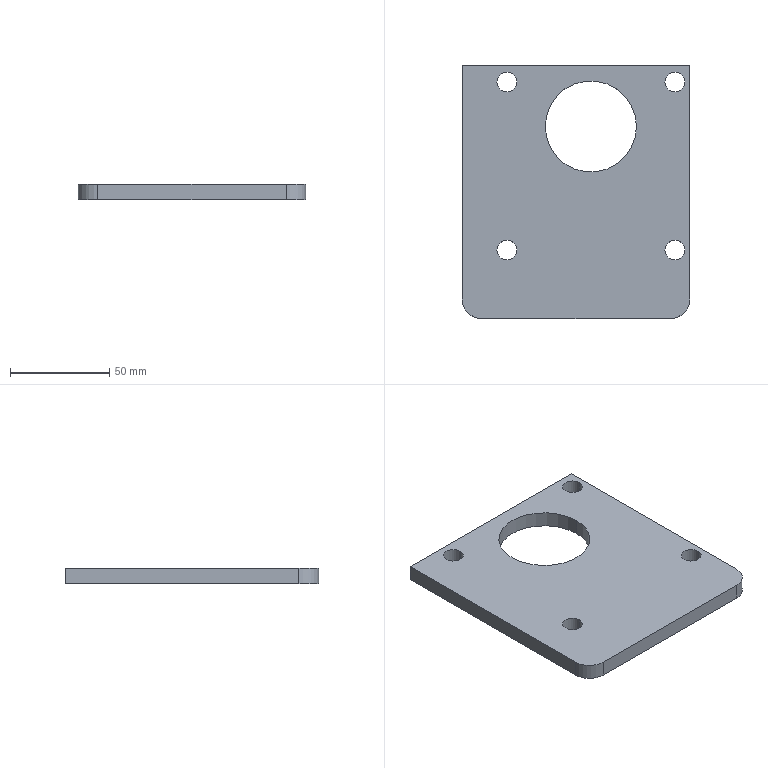Part | SolidWorks | features Chamfer 1, Extrusion 1, Fillet 1, HoleWzd 1, ICE 1 | 1 solid | 18 faces | box 115 x 128 x 8 mm | volume 101608 mm3 | cylinder 12 | plane 6 | commonest cylinder face diameters 10 x8 20 x2 46 x2
STEP:
#1=CARTESIAN_POINT('',(30.5,33.074,-4.));
#2=VERTEX_POINT('',#1);
#3=CARTESIAN_POINT('',(-15.5,33.074,-4.));
#4=VERTEX_POINT('',#3);
#5=CARTESIAN_POINT('',(7.5,33.074,-4.));
#6=DIRECTION('',(0.,0.,-1.));
#7=DIRECTION('',(1.,0.,0.));
#8=AXIS2_PLACEMENT_3D('',#5,#6,#7);
#9=CIRCLE('',#8,23.);
#10=EDGE_CURVE('',#2,#4,#9,.T.);
#11=ORIENTED_EDGE('',*,*,#10,.T.);
#12=CARTESIAN_POINT('',(-15.5,33.074,4.));
#13=VERTEX_POINT('',#12);
#14=CARTESIAN_POINT('',(-15.5,33.074,-4.001));
#15=DIRECTION('',(0.,0.,1.));
#16=VECTOR('',#15,1000.);
#17=LINE('',#14,#16);
#18=EDGE_CURVE('',#4,#13,#17,.T.);
#19=ORIENTED_EDGE('',*,*,#18,.T.);
#20=CARTESIAN_POINT('',(30.5,33.074,4.));
#21=VERTEX_POINT('',#20);
#22=CARTESIAN_POINT('',(7.5,33.074,4.));
#23=DIRECTION('',(0.,0.,1.));
#24=DIRECTION('',(1.,0.,0.));
#25=AXIS2_PLACEMENT_3D('',#22,#23,#24);
#26=CIRCLE('',#25,23.);
#27=EDGE_CURVE('',#13,#21,#26,.T.);
#28=ORIENTED_EDGE('',*,*,#27,.T.);
#29=CARTESIAN_POINT('',(30.5,33.074,-4.001));
#30=DIRECTION('',(0.,0.,1.));
#31=VECTOR('',#30,1000.);
#32=LINE('',#29,#31);
#33=EDGE_CURVE('',#2,#21,#32,.T.);
#34=ORIENTED_EDGE('',*,*,#33,.F.);
#35=EDGE_LOOP('',(#11,#19,#28,#34));
#36=FACE_OUTER_BOUND('',#35,.T.);
#37=CARTESIAN_POINT('',(7.5,33.074,-4.001));
#38=DIRECTION('',(0.,0.,1.));
#39=DIRECTION('',(1.,0.,0.));
#40=AXIS2_PLACEMENT_3D('',#37,#38,#39);
#41=CYLINDRICAL_SURFACE('',#40,23.);
#42=ADVANCED_FACE('',(#36),#41,.F.);
#43=CARTESIAN_POINT('',(-39.926,55.5,-4.));
#44=VERTEX_POINT('',#43);
#45=CARTESIAN_POINT('',(-29.926,55.5,-4.));
#46=VERTEX_POINT('',#45);
#47=CARTESIAN_POINT('',(-34.926,55.5,-4.));
#48=DIRECTION('',(0.,0.,1.));
#49=DIRECTION('',(1.,0.,0.));
#50=AXIS2_PLACEMENT_3D('',#47,#48,#49);
#51=CIRCLE('',#50,5.);
#52=EDGE_CURVE('',#44,#46,#51,.T.);
#53=ORIENTED_EDGE('',*,*,#52,.F.);
#54=CARTESIAN_POINT('',(-39.926,55.5,4.));
#55=VERTEX_POINT('',#54);
#56=CARTESIAN_POINT('',(-39.926,55.5,4.));
#57=DIRECTION('',(0.,0.,1.));
#58=VECTOR('',#57,1000.);
#59=LINE('',#56,#58);
#60=EDGE_CURVE('',#44,#55,#59,.T.);
#61=ORIENTED_EDGE('',*,*,#60,.T.);
#62=CARTESIAN_POINT('',(-29.926,55.5,4.));
#63=VERTEX_POINT('',#62);
#64=CARTESIAN_POINT('',(-34.926,55.5,4.));
#65=DIRECTION('',(0.,0.,1.));
#66=DIRECTION('',(1.,0.,0.));
#67=AXIS2_PLACEMENT_3D('',#64,#65,#66);
#68=CIRCLE('',#67,5.);
#69=EDGE_CURVE('',#55,#63,#68,.T.);
#70=ORIENTED_EDGE('',*,*,#69,.T.);
#71=CARTESIAN_POINT('',(-29.926,55.5,4.));
#72=DIRECTION('',(0.,0.,1.));
#73=VECTOR('',#72,1000.);
#74=LINE('',#71,#73);
#75=EDGE_CURVE('',#46,#63,#74,.T.);
#76=ORIENTED_EDGE('',*,*,#75,.F.);
#77=EDGE_LOOP('',(#53,#61,#70,#76));
#78=FACE_OUTER_BOUND('',#77,.T.);
#79=CARTESIAN_POINT('',(-34.926,55.5,4.));
#80=DIRECTION('',(0.,0.,1.));
#81=DIRECTION('',(1.,0.,0.));
#82=AXIS2_PLACEMENT_3D('',#79,#80,#81);
#83=CYLINDRICAL_SURFACE('',#82,5.);
#84=ADVANCED_FACE('',(#78),#83,.F.);
#85=CARTESIAN_POINT('',(44.926,55.5,-4.));
#86=VERTEX_POINT('',#85);
#87=CARTESIAN_POINT('',(54.926,55.5,-4.));
#88=VERTEX_POINT('',#87);
#89=CARTESIAN_POINT('',(49.926,55.5,-4.));
#90=DIRECTION('',(0.,0.,1.));
#91=DIRECTION('',(1.,0.,0.));
#92=AXIS2_PLACEMENT_3D('',#89,#90,#91);
#93=CIRCLE('',#92,5.);
#94=EDGE_CURVE('',#86,#88,#93,.T.);
#95=ORIENTED_EDGE('',*,*,#94,.F.);
#96=CARTESIAN_POINT('',(44.926,55.5,4.));
#97=VERTEX_POINT('',#96);
#98=CARTESIAN_POINT('',(44.926,55.5,4.));
#99=DIRECTION('',(0.,0.,1.));
#100=VECTOR('',#99,1000.);
#101=LINE('',#98,#100);
#102=EDGE_CURVE('',#86,#97,#101,.T.);
#103=ORIENTED_EDGE('',*,*,#102,.T.);
#104=CARTESIAN_POINT('',(54.926,55.5,4.));
#105=VERTEX_POINT('',#104);
#106=CARTESIAN_POINT('',(49.926,55.5,4.));
#107=DIRECTION('',(0.,0.,1.));
#108=DIRECTION('',(1.,0.,0.));
#109=AXIS2_PLACEMENT_3D('',#106,#107,#108);
#110=CIRCLE('',#109,5.);
#111=EDGE_CURVE('',#97,#105,#110,.T.);
#112=ORIENTED_EDGE('',*,*,#111,.T.);
#113=CARTESIAN_POINT('',(54.926,55.5,4.));
#114=DIRECTION('',(0.,0.,1.));
#115=VECTOR('',#114,1000.);
#116=LINE('',#113,#115);
#117=EDGE_CURVE('',#88,#105,#116,.T.);
#118=ORIENTED_EDGE('',*,*,#117,.F.);
#119=EDGE_LOOP('',(#95,#103,#112,#118));
#120=FACE_OUTER_BOUND('',#119,.T.);
#121=CARTESIAN_POINT('',(49.926,55.5,4.));
#122=DIRECTION('',(0.,0.,1.));
#123=DIRECTION('',(1.,0.,0.));
#124=AXIS2_PLACEMENT_3D('',#121,#122,#123);
#125=CYLINDRICAL_SURFACE('',#124,5.);
#126=ADVANCED_FACE('',(#120),#125,.F.);
#127=CARTESIAN_POINT('',(44.926,-29.353,-4.));
#128=VERTEX_POINT('',#127);
#129=CARTESIAN_POINT('',(54.926,-29.353,-4.));
#130=VERTEX_POINT('',#129);
#131=CARTESIAN_POINT('',(49.926,-29.353,-4.));
#132=DIRECTION('',(0.,0.,1.));
#133=DIRECTION('',(1.,0.,0.));
#134=AXIS2_PLACEMENT_3D('',#131,#132,#133);
#135=CIRCLE('',#134,5.);
#136=EDGE_CURVE('',#128,#130,#135,.T.);
#137=ORIENTED_EDGE('',*,*,#136,.F.);
#138=CARTESIAN_POINT('',(44.926,-29.353,4.));
#139=VERTEX_POINT('',#138);
#140=CARTESIAN_POINT('',(44.926,-29.353,4.));
#141=DIRECTION('',(0.,0.,1.));
#142=VECTOR('',#141,1000.);
#143=LINE('',#140,#142);
#144=EDGE_CURVE('',#128,#139,#143,.T.);
#145=ORIENTED_EDGE('',*,*,#144,.T.);
#146=CARTESIAN_POINT('',(54.926,-29.353,4.));
#147=VERTEX_POINT('',#146);
#148=CARTESIAN_POINT('',(49.926,-29.353,4.));
#149=DIRECTION('',(0.,0.,1.));
#150=DIRECTION('',(1.,0.,0.));
#151=AXIS2_PLACEMENT_3D('',#148,#149,#150);
#152=CIRCLE('',#151,5.);
#153=EDGE_CURVE('',#139,#147,#152,.T.);
#154=ORIENTED_EDGE('',*,*,#153,.T.);
#155=CARTESIAN_POINT('',(54.926,-29.353,4.));
#156=DIRECTION('',(0.,0.,1.));
#157=VECTOR('',#156,1000.);
#158=LINE('',#155,#157);
#159=EDGE_CURVE('',#130,#147,#158,.T.);
#160=ORIENTED_EDGE('',*,*,#159,.F.);
#161=EDGE_LOOP('',(#137,#145,#154,#160));
#162=FACE_OUTER_BOUND('',#161,.T.);
#163=CARTESIAN_POINT('',(49.926,-29.353,4.));
#164=DIRECTION('',(0.,0.,1.));
#165=DIRECTION('',(1.,0.,0.));
#166=AXIS2_PLACEMENT_3D('',#163,#164,#165);
#167=CYLINDRICAL_SURFACE('',#166,5.);
#168=ADVANCED_FACE('',(#162),#167,.F.);
#169=CARTESIAN_POINT('',(-39.926,-29.353,-4.));
#170=VERTEX_POINT('',#169);
#171=CARTESIAN_POINT('',(-29.926,-29.353,-4.));
#172=VERTEX_POINT('',#171);
#173=CARTESIAN_POINT('',(-34.926,-29.353,-4.));
#174=DIRECTION('',(0.,0.,1.));
#175=DIRECTION('',(1.,0.,0.));
#176=AXIS2_PLACEMENT_3D('',#173,#174,#175);
#177=CIRCLE('',#176,5.);
#178=EDGE_CURVE('',#170,#172,#177,.T.);
#179=ORIENTED_EDGE('',*,*,#178,.F.);
#180=CARTESIAN_POINT('',(-39.926,-29.353,4.));
#181=VERTEX_POINT('',#180);
#182=CARTESIAN_POINT('',(-39.926,-29.353,4.));
#183=DIRECTION('',(0.,0.,1.));
#184=VECTOR('',#183,1000.);
#185=LINE('',#182,#184);
#186=EDGE_CURVE('',#170,#181,#185,.T.);
#187=ORIENTED_EDGE('',*,*,#186,.T.);
#188=CARTESIAN_POINT('',(-29.926,-29.353,4.));
#189=VERTEX_POINT('',#188);
#190=CARTESIAN_POINT('',(-34.926,-29.353,4.));
#191=DIRECTION('',(0.,0.,1.));
#192=DIRECTION('',(1.,0.,0.));
#193=AXIS2_PLACEMENT_3D('',#190,#191,#192);
#194=CIRCLE('',#193,5.);
#195=EDGE_CURVE('',#181,#189,#194,.T.);
#196=ORIENTED_EDGE('',*,*,#195,.T.);
#197=CARTESIAN_POINT('',(-29.926,-29.353,4.));
#198=DIRECTION('',(0.,0.,1.));
#199=VECTOR('',#198,1000.);
#200=LINE('',#197,#199);
#201=EDGE_CURVE('',#172,#189,#200,.T.);
#202=ORIENTED_EDGE('',*,*,#201,.F.);
#203=EDGE_LOOP('',(#179,#187,#196,#202));
#204=FACE_OUTER_BOUND('',#203,.T.);
#205=CARTESIAN_POINT('',(-34.926,-29.353,4.));
#206=DIRECTION('',(0.,0.,1.));
#207=DIRECTION('',(1.,0.,0.));
#208=AXIS2_PLACEMENT_3D('',#205,#206,#207);
#209=CYLINDRICAL_SURFACE('',#208,5.);
#210=ADVANCED_FACE('',(#204),#209,.F.);
#211=CARTESIAN_POINT('',(-57.5,64.,-4.));
#212=VERTEX_POINT('',#211);
#213=CARTESIAN_POINT('',(-57.5,-54.,-4.));
#214=VERTEX_POINT('',#213);
#215=CARTESIAN_POINT('',(-57.5,-64.,-4.));
#216=DIRECTION('',(0.,-1.,0.));
#217=VECTOR('',#216,1000.);
#218=LINE('',#215,#217);
#219=EDGE_CURVE('',#212,#214,#218,.T.);
#220=ORIENTED_EDGE('',*,*,#219,.T.);
#221=CARTESIAN_POINT('',(-57.5,-54.,4.));
#222=VERTEX_POINT('',#221);
#223=CARTESIAN_POINT('',(-57.5,-54.,4.));
#224=DIRECTION('',(0.,0.,1.));
#225=VECTOR('',#224,1000.);
#226=LINE('',#223,#225);
#227=EDGE_CURVE('',#214,#222,#226,.T.);
#228=ORIENTED_EDGE('',*,*,#227,.T.);
#229=CARTESIAN_POINT('',(-57.5,64.,4.));
#230=VERTEX_POINT('',#229);
#231=CARTESIAN_POINT('',(-57.5,-64.,4.));
#232=DIRECTION('',(0.,-1.,0.));
#233=VECTOR('',#232,1000.);
#234=LINE('',#231,#233);
#235=EDGE_CURVE('',#230,#222,#234,.T.);
#236=ORIENTED_EDGE('',*,*,#235,.F.);
#237=CARTESIAN_POINT('',(-57.5,64.,4.));
#238=DIRECTION('',(0.,0.,-1.));
#239=VECTOR('',#238,1000.);
#240=LINE('',#237,#239);
#241=EDGE_CURVE('',#230,#212,#240,.T.);
#242=ORIENTED_EDGE('',*,*,#241,.T.);
#243=EDGE_LOOP('',(#220,#228,#236,#242));
#244=FACE_OUTER_BOUND('',#243,.T.);
#245=CARTESIAN_POINT('',(-57.5,-64.,4.));
#246=DIRECTION('',(1.,0.,0.));
#247=DIRECTION('',(0.,0.,-1.));
#248=AXIS2_PLACEMENT_3D('',#245,#246,#247);
#249=PLANE('',#248);
#250=ADVANCED_FACE('',(#244),#249,.F.);
#251=CARTESIAN_POINT('',(-47.5,-64.,-4.));
#252=VERTEX_POINT('',#251);
#253=CARTESIAN_POINT('',(47.5,-64.,-4.));
#254=VERTEX_POINT('',#253);
#255=CARTESIAN_POINT('',(57.5,-64.,-4.));
#256=DIRECTION('',(1.,0.,0.));
#257=VECTOR('',#256,1000.);
#258=LINE('',#255,#257);
#259=EDGE_CURVE('',#252,#254,#258,.T.);
#260=ORIENTED_EDGE('',*,*,#259,.T.);
#261=CARTESIAN_POINT('',(47.5,-64.,4.));
#262=VERTEX_POINT('',#261);
#263=CARTESIAN_POINT('',(47.5,-64.,4.));
#264=DIRECTION('',(0.,0.,1.));
#265=VECTOR('',#264,1000.);
#266=LINE('',#263,#265);
#267=EDGE_CURVE('',#254,#262,#266,.T.);
#268=ORIENTED_EDGE('',*,*,#267,.T.);
#269=CARTESIAN_POINT('',(-47.5,-64.,4.));
#270=VERTEX_POINT('',#269);
#271=CARTESIAN_POINT('',(57.5,-64.,4.));
#272=DIRECTION('',(1.,0.,0.));
#273=VECTOR('',#272,1000.);
#274=LINE('',#271,#273);
#275=EDGE_CURVE('',#270,#262,#274,.T.);
#276=ORIENTED_EDGE('',*,*,#275,.F.);
#277=CARTESIAN_POINT('',(-47.5,-64.,4.));
#278=DIRECTION('',(0.,0.,-1.));
#279=VECTOR('',#278,1000.);
#280=LINE('',#277,#279);
#281=EDGE_CURVE('',#270,#252,#280,.T.);
#282=ORIENTED_EDGE('',*,*,#281,.T.);
#283=EDGE_LOOP('',(#260,#268,#276,#282));
#284=FACE_OUTER_BOUND('',#283,.T.);
#285=CARTESIAN_POINT('',(57.5,-64.,4.));
#286=DIRECTION('',(0.,1.,0.));
#287=DIRECTION('',(-1.,0.,0.));
#288=AXIS2_PLACEMENT_3D('',#285,#286,#287);
#289=PLANE('',#288);
#290=ADVANCED_FACE('',(#284),#289,.F.);
#291=CARTESIAN_POINT('',(57.5,-54.,4.));
#292=VERTEX_POINT('',#291);
#293=CARTESIAN_POINT('',(57.5,64.,4.));
#294=VERTEX_POINT('',#293);
#295=CARTESIAN_POINT('',(57.5,-64.,4.));
#296=DIRECTION('',(0.,1.,0.));
#297=VECTOR('',#296,1000.);
#298=LINE('',#295,#297);
#299=EDGE_CURVE('',#292,#294,#298,.T.);
#300=ORIENTED_EDGE('',*,*,#299,.F.);
#301=CARTESIAN_POINT('',(57.5,-54.,-4.));
#302=VERTEX_POINT('',#301);
#303=CARTESIAN_POINT('',(57.5,-54.,4.));
#304=DIRECTION('',(0.,0.,-1.));
#305=VECTOR('',#304,1000.);
#306=LINE('',#303,#305);
#307=EDGE_CURVE('',#292,#302,#306,.T.);
#308=ORIENTED_EDGE('',*,*,#307,.T.);
#309=CARTESIAN_POINT('',(57.5,64.,-4.));
#310=VERTEX_POINT('',#309);
#311=CARTESIAN_POINT('',(57.5,-64.,-4.));
#312=DIRECTION('',(0.,1.,0.));
#313=VECTOR('',#312,1000.);
#314=LINE('',#311,#313);
#315=EDGE_CURVE('',#302,#310,#314,.T.);
#316=ORIENTED_EDGE('',*,*,#315,.T.);
#317=CARTESIAN_POINT('',(57.5,64.,4.));
#318=DIRECTION('',(0.,0.,-1.));
#319=VECTOR('',#318,1000.);
#320=LINE('',#317,#319);
#321=EDGE_CURVE('',#294,#310,#320,.T.);
#322=ORIENTED_EDGE('',*,*,#321,.F.);
#323=EDGE_LOOP('',(#300,#308,#316,#322));
#324=FACE_OUTER_BOUND('',#323,.T.);
#325=CARTESIAN_POINT('',(57.5,-64.,4.));
#326=DIRECTION('',(-1.,0.,0.));
#327=DIRECTION('',(0.,0.,1.));
#328=AXIS2_PLACEMENT_3D('',#325,#326,#327);
#329=PLANE('',#328);
#330=ADVANCED_FACE('',(#324),#329,.F.);
#331=CARTESIAN_POINT('',(57.5,64.,-4.));
#332=DIRECTION('',(-1.,0.,0.));
#333=VECTOR('',#332,1000.);
#334=LINE('',#331,#333);
#335=EDGE_CURVE('',#310,#212,#334,.T.);
#336=ORIENTED_EDGE('',*,*,#335,.T.);
#337=ORIENTED_EDGE('',*,*,#241,.F.);
#338=CARTESIAN_POINT('',(57.5,64.,4.));
#339=DIRECTION('',(-1.,0.,0.));
#340=VECTOR('',#339,1000.);
#341=LINE('',#338,#340);
#342=EDGE_CURVE('',#294,#230,#341,.T.);
#343=ORIENTED_EDGE('',*,*,#342,.F.);
#344=ORIENTED_EDGE('',*,*,#321,.T.);
#345=EDGE_LOOP('',(#336,#337,#343,#344));
#346=FACE_OUTER_BOUND('',#345,.T.);
#347=CARTESIAN_POINT('',(57.5,64.,4.));
#348=DIRECTION('',(0.,-1.,0.));
#349=DIRECTION('',(1.,0.,0.));
#350=AXIS2_PLACEMENT_3D('',#347,#348,#349);
#351=PLANE('',#350);
#352=ADVANCED_FACE('',(#346),#351,.F.);
#353=CARTESIAN_POINT('',(7.5,33.074,4.));
#354=DIRECTION('',(0.,0.,1.));
#355=DIRECTION('',(1.,0.,0.));
#356=AXIS2_PLACEMENT_3D('',#353,#354,#355);
#357=CIRCLE('',#356,23.);
#358=EDGE_CURVE('',#21,#13,#357,.T.);
#359=ORIENTED_EDGE('',*,*,#358,.F.);
#360=ORIENTED_EDGE('',*,*,#27,.F.);
#361=EDGE_LOOP('',(#359,#360));
#362=FACE_BOUND('',#361,.T.);
#363=CARTESIAN_POINT('',(-34.926,55.5,4.));
#364=DIRECTION('',(0.,0.,1.));
#365=DIRECTION('',(1.,0.,0.));
#366=AXIS2_PLACEMENT_3D('',#363,#364,#365);
#367=CIRCLE('',#366,5.);
#368=EDGE_CURVE('',#63,#55,#367,.T.);
#369=ORIENTED_EDGE('',*,*,#368,.F.);
#370=ORIENTED_EDGE('',*,*,#69,.F.);
#371=EDGE_LOOP('',(#369,#370));
#372=FACE_BOUND('',#371,.T.);
#373=CARTESIAN_POINT('',(49.926,55.5,4.));
#374=DIRECTION('',(0.,0.,1.));
#375=DIRECTION('',(1.,0.,0.));
#376=AXIS2_PLACEMENT_3D('',#373,#374,#375);
#377=CIRCLE('',#376,5.);
#378=EDGE_CURVE('',#105,#97,#377,.T.);
#379=ORIENTED_EDGE('',*,*,#378,.F.);
#380=ORIENTED_EDGE('',*,*,#111,.F.);
#381=EDGE_LOOP('',(#379,#380));
#382=FACE_BOUND('',#381,.T.);
#383=CARTESIAN_POINT('',(49.926,-29.353,4.));
#384=DIRECTION('',(0.,0.,1.));
#385=DIRECTION('',(1.,0.,0.));
#386=AXIS2_PLACEMENT_3D('',#383,#384,#385);
#387=CIRCLE('',#386,5.);
#388=EDGE_CURVE('',#147,#139,#387,.T.);
#389=ORIENTED_EDGE('',*,*,#388,.F.);
#390=ORIENTED_EDGE('',*,*,#153,.F.);
#391=EDGE_LOOP('',(#389,#390));
#392=FACE_BOUND('',#391,.T.);
#393=CARTESIAN_POINT('',(-34.926,-29.353,4.));
#394=DIRECTION('',(0.,0.,1.));
#395=DIRECTION('',(1.,0.,0.));
#396=AXIS2_PLACEMENT_3D('',#393,#394,#395);
#397=CIRCLE('',#396,5.);
#398=EDGE_CURVE('',#189,#181,#397,.T.);
#399=ORIENTED_EDGE('',*,*,#398,.F.);
#400=ORIENTED_EDGE('',*,*,#195,.F.);
#401=EDGE_LOOP('',(#399,#400));
#402=FACE_BOUND('',#401,.T.);
#403=ORIENTED_EDGE('',*,*,#275,.T.);
#404=CARTESIAN_POINT('',(47.5,-54.,4.));
#405=DIRECTION('',(0.,0.,1.));
#406=DIRECTION('',(1.,0.,0.));
#407=AXIS2_PLACEMENT_3D('',#404,#405,#406);
#408=CIRCLE('',#407,10.);
#409=EDGE_CURVE('',#262,#292,#408,.T.);
#410=ORIENTED_EDGE('',*,*,#409,.T.);
#411=ORIENTED_EDGE('',*,*,#299,.T.);
#412=ORIENTED_EDGE('',*,*,#342,.T.);
#413=ORIENTED_EDGE('',*,*,#235,.T.);
#414=CARTESIAN_POINT('',(-47.5,-54.,4.));
#415=DIRECTION('',(0.,0.,1.));
#416=DIRECTION('',(1.,0.,0.));
#417=AXIS2_PLACEMENT_3D('',#414,#415,#416);
#418=CIRCLE('',#417,10.);
#419=EDGE_CURVE('',#222,#270,#418,.T.);
#420=ORIENTED_EDGE('',*,*,#419,.T.);
#421=EDGE_LOOP('',(#403,#410,#411,#412,#413,#420));
#422=FACE_OUTER_BOUND('',#421,.T.);
#423=CARTESIAN_POINT('',(0.,0.,4.));
#424=DIRECTION('',(0.,0.,1.));
#425=DIRECTION('',(1.,0.,0.));
#426=AXIS2_PLACEMENT_3D('',#423,#424,#425);
#427=PLANE('',#426);
#428=ADVANCED_FACE('',(#362,#372,#382,#392,#402,#422),#427,.T.);
#429=ORIENTED_EDGE('',*,*,#10,.F.);
#430=CARTESIAN_POINT('',(7.5,33.074,-4.));
#431=DIRECTION('',(0.,0.,-1.));
#432=DIRECTION('',(1.,0.,0.));
#433=AXIS2_PLACEMENT_3D('',#430,#431,#432);
#434=CIRCLE('',#433,23.);
#435=EDGE_CURVE('',#4,#2,#434,.T.);
#436=ORIENTED_EDGE('',*,*,#435,.F.);
#437=EDGE_LOOP('',(#429,#436));
#438=FACE_BOUND('',#437,.T.);
#439=CARTESIAN_POINT('',(-34.926,55.5,-4.));
#440=DIRECTION('',(0.,0.,1.));
#441=DIRECTION('',(1.,0.,0.));
#442=AXIS2_PLACEMENT_3D('',#439,#440,#441);
#443=CIRCLE('',#442,5.);
#444=EDGE_CURVE('',#46,#44,#443,.T.);
#445=ORIENTED_EDGE('',*,*,#444,.T.);
#446=ORIENTED_EDGE('',*,*,#52,.T.);
#447=EDGE_LOOP('',(#445,#446));
#448=FACE_BOUND('',#447,.T.);
#449=CARTESIAN_POINT('',(49.926,55.5,-4.));
#450=DIRECTION('',(0.,0.,1.));
#451=DIRECTION('',(1.,0.,0.));
#452=AXIS2_PLACEMENT_3D('',#449,#450,#451);
#453=CIRCLE('',#452,5.);
#454=EDGE_CURVE('',#88,#86,#453,.T.);
#455=ORIENTED_EDGE('',*,*,#454,.T.);
#456=ORIENTED_EDGE('',*,*,#94,.T.);
#457=EDGE_LOOP('',(#455,#456));
#458=FACE_BOUND('',#457,.T.);
#459=CARTESIAN_POINT('',(49.926,-29.353,-4.));
#460=DIRECTION('',(0.,0.,1.));
#461=DIRECTION('',(1.,0.,0.));
#462=AXIS2_PLACEMENT_3D('',#459,#460,#461);
#463=CIRCLE('',#462,5.);
#464=EDGE_CURVE('',#130,#128,#463,.T.);
#465=ORIENTED_EDGE('',*,*,#464,.T.);
#466=ORIENTED_EDGE('',*,*,#136,.T.);
#467=EDGE_LOOP('',(#465,#466));
#468=FACE_BOUND('',#467,.T.);
#469=CARTESIAN_POINT('',(-34.926,-29.353,-4.));
#470=DIRECTION('',(0.,0.,1.));
#471=DIRECTION('',(1.,0.,0.));
#472=AXIS2_PLACEMENT_3D('',#469,#470,#471);
#473=CIRCLE('',#472,5.);
#474=EDGE_CURVE('',#172,#170,#473,.T.);
#475=ORIENTED_EDGE('',*,*,#474,.T.);
#476=ORIENTED_EDGE('',*,*,#178,.T.);
#477=EDGE_LOOP('',(#475,#476));
#478=FACE_BOUND('',#477,.T.);
#479=ORIENTED_EDGE('',*,*,#315,.F.);
#480=CARTESIAN_POINT('',(47.5,-54.,-4.));
#481=DIRECTION('',(0.,0.,-1.));
#482=DIRECTION('',(1.,0.,0.));
#483=AXIS2_PLACEMENT_3D('',#480,#481,#482);
#484=CIRCLE('',#483,10.);
#485=EDGE_CURVE('',#302,#254,#484,.T.);
#486=ORIENTED_EDGE('',*,*,#485,.T.);
#487=ORIENTED_EDGE('',*,*,#259,.F.);
#488=CARTESIAN_POINT('',(-47.5,-54.,-4.));
#489=DIRECTION('',(0.,0.,-1.));
#490=DIRECTION('',(1.,0.,0.));
#491=AXIS2_PLACEMENT_3D('',#488,#489,#490);
#492=CIRCLE('',#491,10.);
#493=EDGE_CURVE('',#252,#214,#492,.T.);
#494=ORIENTED_EDGE('',*,*,#493,.T.);
#495=ORIENTED_EDGE('',*,*,#219,.F.);
#496=ORIENTED_EDGE('',*,*,#335,.F.);
#497=EDGE_LOOP('',(#479,#486,#487,#494,#495,#496));
#498=FACE_OUTER_BOUND('',#497,.T.);
#499=CARTESIAN_POINT('',(0.,0.,-4.));
#500=DIRECTION('',(0.,0.,1.));
#501=DIRECTION('',(1.,0.,0.));
#502=AXIS2_PLACEMENT_3D('',#499,#500,#501);
#503=PLANE('',#502);
#504=ADVANCED_FACE('',(#438,#448,#458,#468,#478,#498),#503,.F.);
#505=ORIENTED_EDGE('',*,*,#186,.F.);
#506=ORIENTED_EDGE('',*,*,#474,.F.);
#507=ORIENTED_EDGE('',*,*,#201,.T.);
#508=ORIENTED_EDGE('',*,*,#398,.T.);
#509=EDGE_LOOP('',(#505,#506,#507,#508));
#510=FACE_OUTER_BOUND('',#509,.T.);
#511=CARTESIAN_POINT('',(-34.926,-29.353,4.));
#512=DIRECTION('',(0.,0.,1.));
#513=DIRECTION('',(1.,0.,0.));
#514=AXIS2_PLACEMENT_3D('',#511,#512,#513);
#515=CYLINDRICAL_SURFACE('',#514,5.);
#516=ADVANCED_FACE('',(#510),#515,.F.);
#517=ORIENTED_EDGE('',*,*,#144,.F.);
#518=ORIENTED_EDGE('',*,*,#464,.F.);
#519=ORIENTED_EDGE('',*,*,#159,.T.);
#520=ORIENTED_EDGE('',*,*,#388,.T.);
#521=EDGE_LOOP('',(#517,#518,#519,#520));
#522=FACE_OUTER_BOUND('',#521,.T.);
#523=CARTESIAN_POINT('',(49.926,-29.353,4.));
#524=DIRECTION('',(0.,0.,1.));
#525=DIRECTION('',(1.,0.,0.));
#526=AXIS2_PLACEMENT_3D('',#523,#524,#525);
#527=CYLINDRICAL_SURFACE('',#526,5.);
#528=ADVANCED_FACE('',(#522),#527,.F.);
#529=ORIENTED_EDGE('',*,*,#102,.F.);
#530=ORIENTED_EDGE('',*,*,#454,.F.);
#531=ORIENTED_EDGE('',*,*,#117,.T.);
#532=ORIENTED_EDGE('',*,*,#378,.T.);
#533=EDGE_LOOP('',(#529,#530,#531,#532));
#534=FACE_OUTER_BOUND('',#533,.T.);
#535=CARTESIAN_POINT('',(49.926,55.5,4.));
#536=DIRECTION('',(0.,0.,1.));
#537=DIRECTION('',(1.,0.,0.));
#538=AXIS2_PLACEMENT_3D('',#535,#536,#537);
#539=CYLINDRICAL_SURFACE('',#538,5.);
#540=ADVANCED_FACE('',(#534),#539,.F.);
#541=ORIENTED_EDGE('',*,*,#60,.F.);
#542=ORIENTED_EDGE('',*,*,#444,.F.);
#543=ORIENTED_EDGE('',*,*,#75,.T.);
#544=ORIENTED_EDGE('',*,*,#368,.T.);
#545=EDGE_LOOP('',(#541,#542,#543,#544));
#546=FACE_OUTER_BOUND('',#545,.T.);
#547=CARTESIAN_POINT('',(-34.926,55.5,4.));
#548=DIRECTION('',(0.,0.,1.));
#549=DIRECTION('',(1.,0.,0.));
#550=AXIS2_PLACEMENT_3D('',#547,#548,#549);
#551=CYLINDRICAL_SURFACE('',#550,5.);
#552=ADVANCED_FACE('',(#546),#551,.F.);
#553=ORIENTED_EDGE('',*,*,#409,.F.);
#554=ORIENTED_EDGE('',*,*,#267,.F.);
#555=ORIENTED_EDGE('',*,*,#485,.F.);
#556=ORIENTED_EDGE('',*,*,#307,.F.);
#557=EDGE_LOOP('',(#553,#554,#555,#556));
#558=FACE_OUTER_BOUND('',#557,.T.);
#559=CARTESIAN_POINT('',(47.5,-54.,4.));
#560=DIRECTION('',(0.,0.,-1.));
#561=DIRECTION('',(-1.,0.,0.));
#562=AXIS2_PLACEMENT_3D('',#559,#560,#561);
#563=CYLINDRICAL_SURFACE('',#562,10.);
#564=ADVANCED_FACE('',(#558),#563,.T.);
#565=ORIENTED_EDGE('',*,*,#419,.F.);
#566=ORIENTED_EDGE('',*,*,#227,.F.);
#567=ORIENTED_EDGE('',*,*,#493,.F.);
#568=ORIENTED_EDGE('',*,*,#281,.F.);
#569=EDGE_LOOP('',(#565,#566,#567,#568));
#570=FACE_OUTER_BOUND('',#569,.T.);
#571=CARTESIAN_POINT('',(-47.5,-54.,4.));
#572=DIRECTION('',(0.,0.,-1.));
#573=DIRECTION('',(-1.,0.,0.));
#574=AXIS2_PLACEMENT_3D('',#571,#572,#573);
#575=CYLINDRICAL_SURFACE('',#574,10.);
#576=ADVANCED_FACE('',(#570),#575,.T.);
#577=ORIENTED_EDGE('',*,*,#18,.F.);
#578=ORIENTED_EDGE('',*,*,#435,.T.);
#579=ORIENTED_EDGE('',*,*,#33,.T.);
#580=ORIENTED_EDGE('',*,*,#358,.T.);
#581=EDGE_LOOP('',(#577,#578,#579,#580));
#582=FACE_OUTER_BOUND('',#581,.T.);
#583=CARTESIAN_POINT('',(7.5,33.074,-4.001));
#584=DIRECTION('',(0.,0.,1.));
#585=DIRECTION('',(1.,0.,0.));
#586=AXIS2_PLACEMENT_3D('',#583,#584,#585);
#587=CYLINDRICAL_SURFACE('',#586,23.);
#588=ADVANCED_FACE('',(#582),#587,.F.);
#589=CLOSED_SHELL('',(#42,#84,#126,#168,#210,#250,#290,#330,#352,#428,#504,#516,#528,#540,#552,#564,#576,#588));
#590=MANIFOLD_SOLID_BREP('',#589);
#591=CARTESIAN_POINT('',(0.,0.,0.));
#592=DIRECTION('',(0.,0.,1.));
#593=DIRECTION('',(1.,0.,0.));
#594=AXIS2_PLACEMENT_3D('',#591,#592,#593);
#595=(LENGTH_UNIT()NAMED_UNIT(*)SI_UNIT(.MILLI.,.METRE.));
#596=UNCERTAINTY_MEASURE_WITH_UNIT(LENGTH_MEASURE(0.00001),#595,'','');
#597=(NAMED_UNIT(*)PLANE_ANGLE_UNIT()SI_UNIT($,.RADIAN.));
#598=(NAMED_UNIT(*)SI_UNIT($,.STERADIAN.)SOLID_ANGLE_UNIT());
#599=(GEOMETRIC_REPRESENTATION_CONTEXT(3)GLOBAL_UNCERTAINTY_ASSIGNED_CONTEXT((#596))GLOBAL_UNIT_ASSIGNED_CONTEXT((#595,#597,#598))REPRESENTATION_CONTEXT('',''));
#600=ADVANCED_BREP_SHAPE_REPRESENTATION('',(#590,#594),#599);